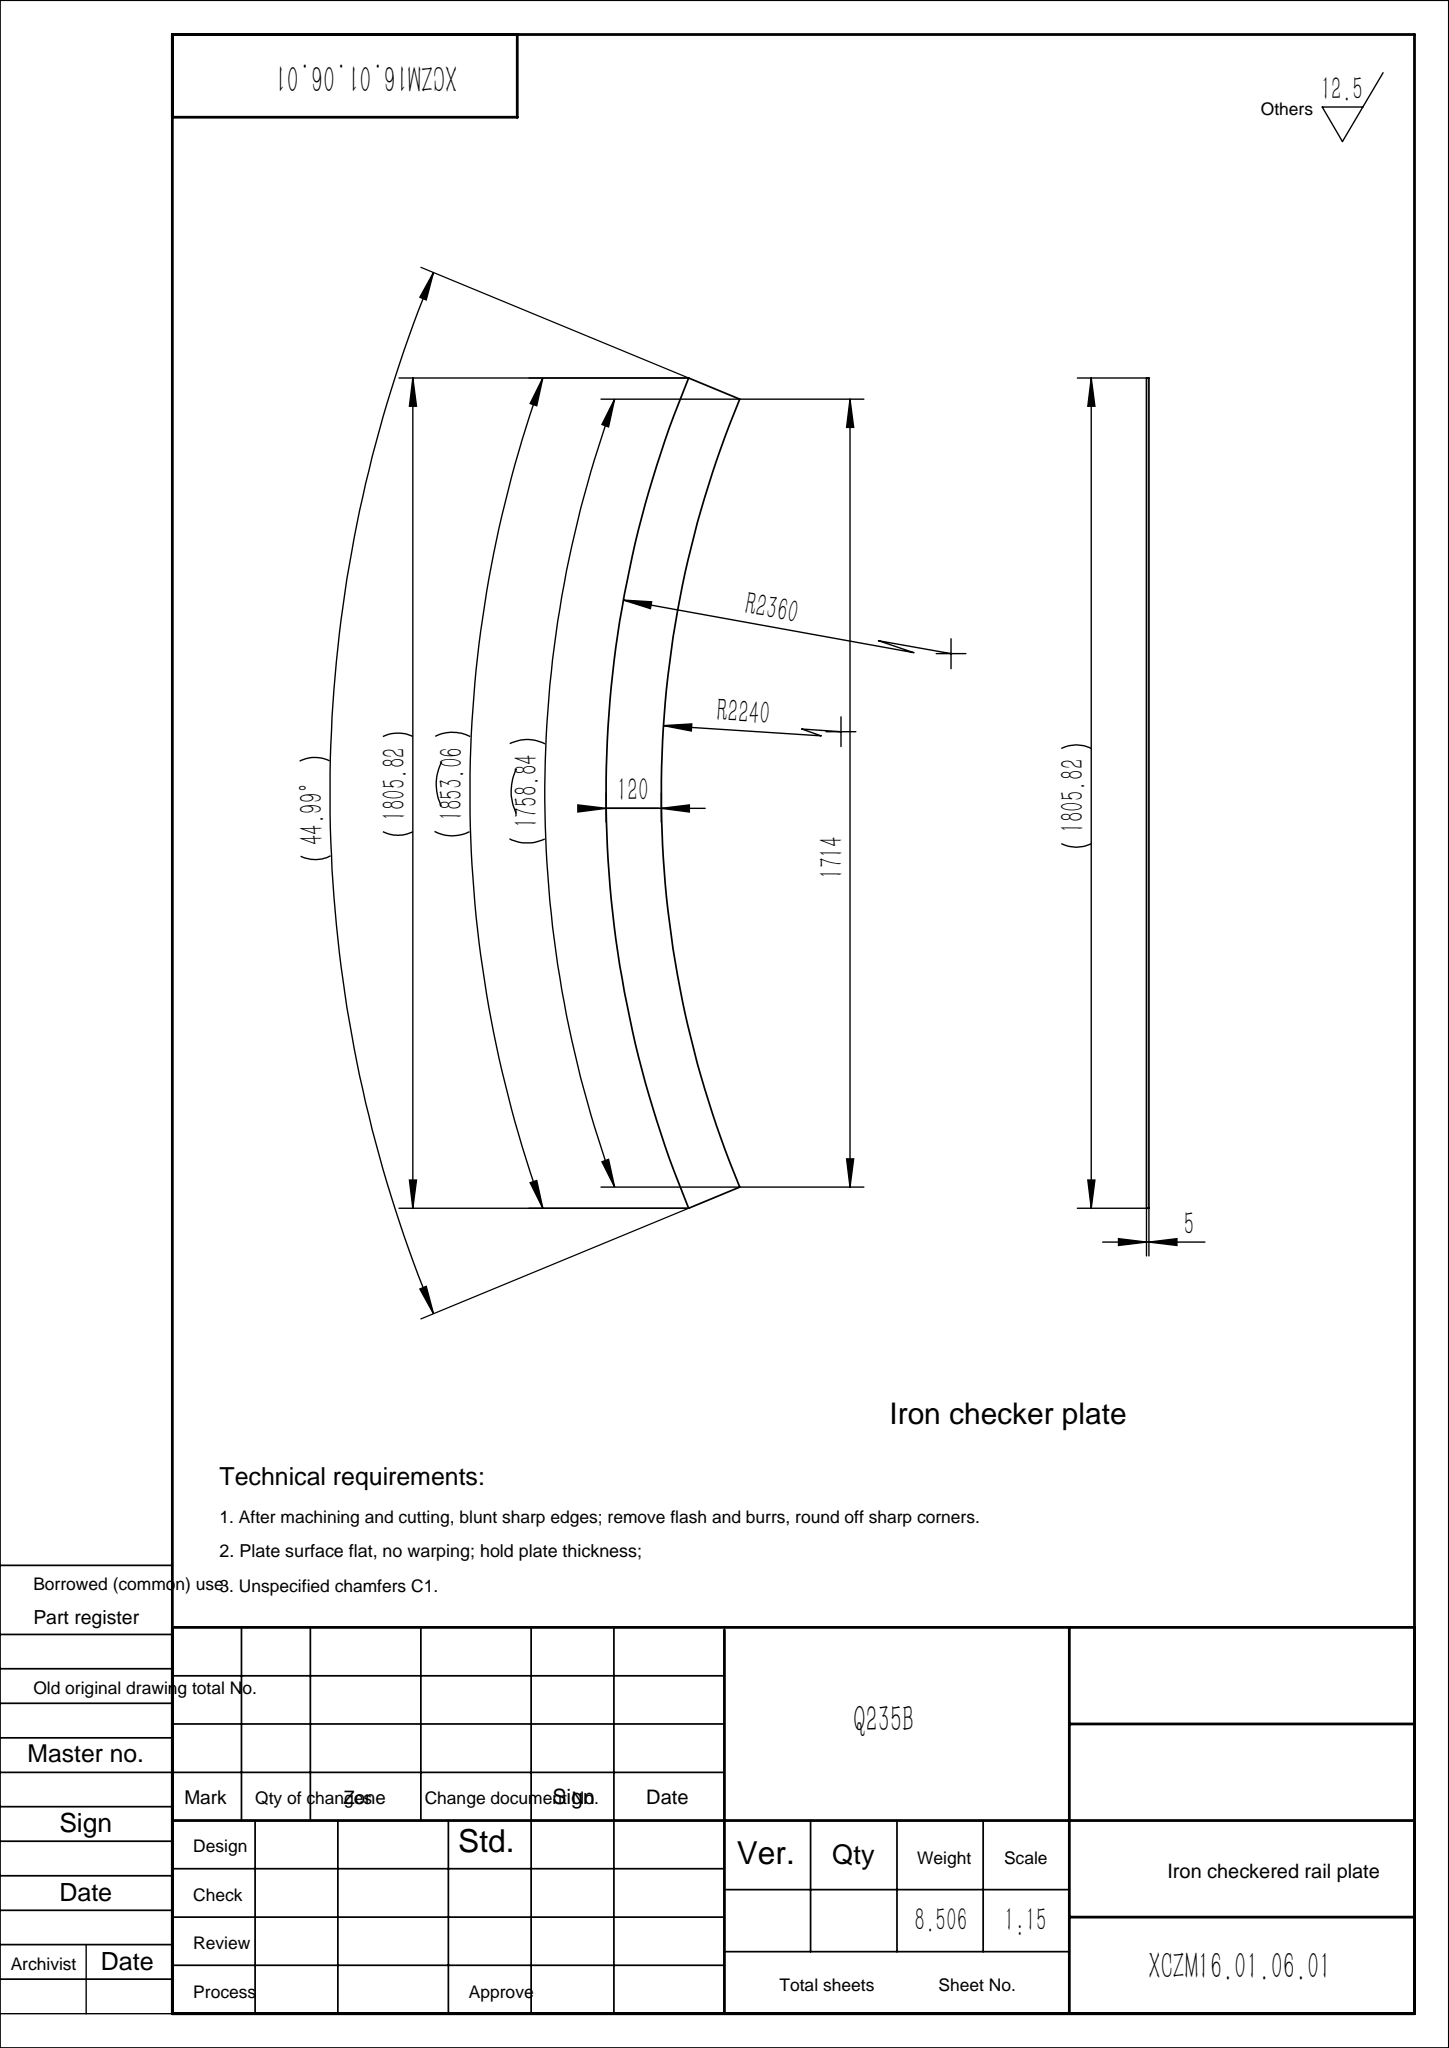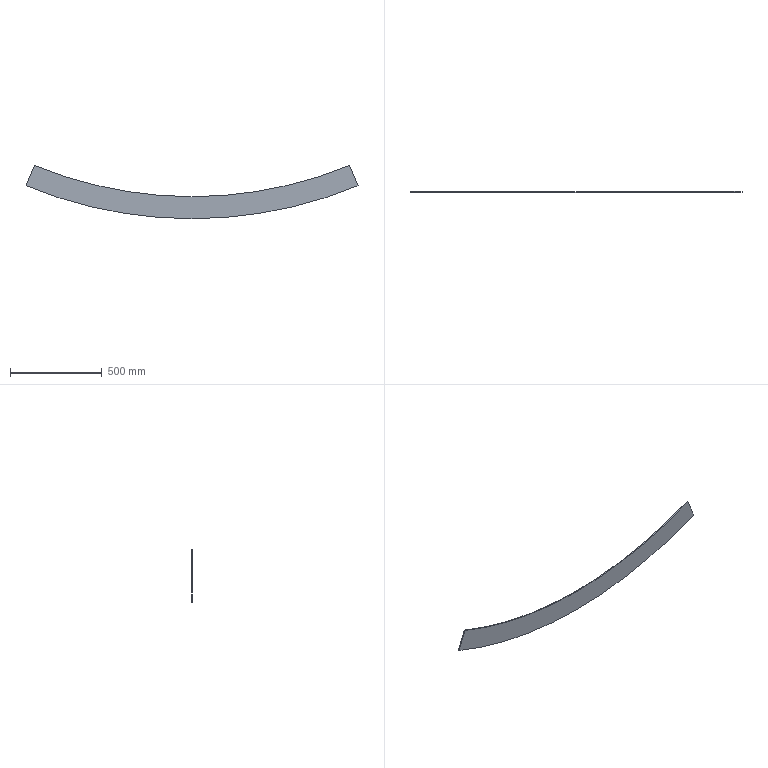Part | SolidWorks | features Extrusion 1 | 1 solid | 8 faces | box 1806 x 5 x 290.423 mm | volume 1083568 mm3 | cylinder 4 | plane 4 | commonest cylinder face diameters 4480 x2 4720 x2
STEP:
#1=CARTESIAN_POINT('',(0.,5.,-2360.));
#2=VERTEX_POINT('',#1);
#3=CARTESIAN_POINT('',(-902.911,5.,-2180.448));
#4=VERTEX_POINT('',#3);
#5=CARTESIAN_POINT('',(0.,5.,0.));
#6=DIRECTION('',(0.,1.,0.));
#7=DIRECTION('',(0.,0.,1.));
#8=AXIS2_PLACEMENT_3D('',#5,#6,#7);
#9=CIRCLE('',#8,2360.);
#10=EDGE_CURVE('',#2,#4,#9,.T.);
#11=ORIENTED_EDGE('',*,*,#10,.F.);
#12=CARTESIAN_POINT('',(0.,0.,-2360.));
#13=VERTEX_POINT('',#12);
#14=CARTESIAN_POINT('',(0.,5.,-2360.));
#15=DIRECTION('',(0.,-1.,0.));
#16=VECTOR('',#15,1000.);
#17=LINE('',#14,#16);
#18=EDGE_CURVE('',#2,#13,#17,.T.);
#19=ORIENTED_EDGE('',*,*,#18,.T.);
#20=CARTESIAN_POINT('',(-902.911,0.,-2180.448));
#21=VERTEX_POINT('',#20);
#22=CARTESIAN_POINT('',(0.,0.,0.));
#23=DIRECTION('',(0.,1.,0.));
#24=DIRECTION('',(0.,0.,1.));
#25=AXIS2_PLACEMENT_3D('',#22,#23,#24);
#26=CIRCLE('',#25,2360.);
#27=EDGE_CURVE('',#13,#21,#26,.T.);
#28=ORIENTED_EDGE('',*,*,#27,.T.);
#29=CARTESIAN_POINT('',(-902.911,5.,-2180.448));
#30=DIRECTION('',(0.,-1.,0.));
#31=VECTOR('',#30,1000.);
#32=LINE('',#29,#31);
#33=EDGE_CURVE('',#4,#21,#32,.T.);
#34=ORIENTED_EDGE('',*,*,#33,.F.);
#35=EDGE_LOOP('',(#11,#19,#28,#34));
#36=FACE_OUTER_BOUND('',#35,.T.);
#37=CARTESIAN_POINT('',(0.,5.,0.));
#38=DIRECTION('',(0.,-1.,0.));
#39=DIRECTION('',(0.,0.,-1.));
#40=AXIS2_PLACEMENT_3D('',#37,#38,#39);
#41=CYLINDRICAL_SURFACE('',#40,2360.);
#42=ADVANCED_FACE('',(#36),#41,.T.);
#43=CARTESIAN_POINT('',(857.,5.,-2069.577));
#44=VERTEX_POINT('',#43);
#45=CARTESIAN_POINT('',(0.,5.,-2240.));
#46=VERTEX_POINT('',#45);
#47=CARTESIAN_POINT('',(0.,5.,0.));
#48=DIRECTION('',(0.,1.,0.));
#49=DIRECTION('',(0.,0.,1.));
#50=AXIS2_PLACEMENT_3D('',#47,#48,#49);
#51=CIRCLE('',#50,2240.);
#52=EDGE_CURVE('',#44,#46,#51,.T.);
#53=ORIENTED_EDGE('',*,*,#52,.T.);
#54=CARTESIAN_POINT('',(0.,0.,-2240.));
#55=VERTEX_POINT('',#54);
#56=CARTESIAN_POINT('',(0.,5.,-2240.));
#57=DIRECTION('',(0.,-1.,0.));
#58=VECTOR('',#57,1000.);
#59=LINE('',#56,#58);
#60=EDGE_CURVE('',#46,#55,#59,.T.);
#61=ORIENTED_EDGE('',*,*,#60,.T.);
#62=CARTESIAN_POINT('',(857.,0.,-2069.577));
#63=VERTEX_POINT('',#62);
#64=CARTESIAN_POINT('',(0.,0.,0.));
#65=DIRECTION('',(0.,1.,0.));
#66=DIRECTION('',(0.,0.,1.));
#67=AXIS2_PLACEMENT_3D('',#64,#65,#66);
#68=CIRCLE('',#67,2240.);
#69=EDGE_CURVE('',#63,#55,#68,.T.);
#70=ORIENTED_EDGE('',*,*,#69,.F.);
#71=CARTESIAN_POINT('',(857.,5.,-2069.577));
#72=DIRECTION('',(0.,-1.,0.));
#73=VECTOR('',#72,1000.);
#74=LINE('',#71,#73);
#75=EDGE_CURVE('',#44,#63,#74,.T.);
#76=ORIENTED_EDGE('',*,*,#75,.F.);
#77=EDGE_LOOP('',(#53,#61,#70,#76));
#78=FACE_OUTER_BOUND('',#77,.T.);
#79=CARTESIAN_POINT('',(0.,5.,0.));
#80=DIRECTION('',(0.,-1.,0.));
#81=DIRECTION('',(0.,0.,-1.));
#82=AXIS2_PLACEMENT_3D('',#79,#80,#81);
#83=CYLINDRICAL_SURFACE('',#82,2240.);
#84=ADVANCED_FACE('',(#78),#83,.F.);
#85=ORIENTED_EDGE('',*,*,#60,.F.);
#86=CARTESIAN_POINT('',(-857.,5.,-2069.577));
#87=VERTEX_POINT('',#86);
#88=CARTESIAN_POINT('',(0.,5.,0.));
#89=DIRECTION('',(0.,1.,0.));
#90=DIRECTION('',(0.,0.,1.));
#91=AXIS2_PLACEMENT_3D('',#88,#89,#90);
#92=CIRCLE('',#91,2240.);
#93=EDGE_CURVE('',#46,#87,#92,.T.);
#94=ORIENTED_EDGE('',*,*,#93,.T.);
#95=CARTESIAN_POINT('',(-857.,0.,-2069.577));
#96=VERTEX_POINT('',#95);
#97=CARTESIAN_POINT('',(-857.,5.,-2069.577));
#98=DIRECTION('',(0.,-1.,0.));
#99=VECTOR('',#98,1000.);
#100=LINE('',#97,#99);
#101=EDGE_CURVE('',#87,#96,#100,.T.);
#102=ORIENTED_EDGE('',*,*,#101,.T.);
#103=CARTESIAN_POINT('',(0.,0.,0.));
#104=DIRECTION('',(0.,1.,0.));
#105=DIRECTION('',(0.,0.,1.));
#106=AXIS2_PLACEMENT_3D('',#103,#104,#105);
#107=CIRCLE('',#106,2240.);
#108=EDGE_CURVE('',#55,#96,#107,.T.);
#109=ORIENTED_EDGE('',*,*,#108,.F.);
#110=EDGE_LOOP('',(#85,#94,#102,#109));
#111=FACE_OUTER_BOUND('',#110,.T.);
#112=CARTESIAN_POINT('',(0.,5.,0.));
#113=DIRECTION('',(0.,-1.,0.));
#114=DIRECTION('',(0.,0.,-1.));
#115=AXIS2_PLACEMENT_3D('',#112,#113,#114);
#116=CYLINDRICAL_SURFACE('',#115,2240.);
#117=ADVANCED_FACE('',(#111),#116,.F.);
#118=CARTESIAN_POINT('',(902.911,0.,-2180.448));
#119=VERTEX_POINT('',#118);
#120=CARTESIAN_POINT('',(0.,0.,0.));
#121=DIRECTION('',(0.3826,0.,-0.9239));
#122=VECTOR('',#121,1000.);
#123=LINE('',#120,#122);
#124=EDGE_CURVE('',#63,#119,#123,.T.);
#125=ORIENTED_EDGE('',*,*,#124,.T.);
#126=CARTESIAN_POINT('',(902.911,5.,-2180.448));
#127=VERTEX_POINT('',#126);
#128=CARTESIAN_POINT('',(902.911,5.,-2180.448));
#129=DIRECTION('',(0.,-1.,0.));
#130=VECTOR('',#129,1000.);
#131=LINE('',#128,#130);
#132=EDGE_CURVE('',#127,#119,#131,.T.);
#133=ORIENTED_EDGE('',*,*,#132,.F.);
#134=CARTESIAN_POINT('',(0.,5.,0.));
#135=DIRECTION('',(0.3826,0.,-0.9239));
#136=VECTOR('',#135,1000.);
#137=LINE('',#134,#136);
#138=EDGE_CURVE('',#44,#127,#137,.T.);
#139=ORIENTED_EDGE('',*,*,#138,.F.);
#140=ORIENTED_EDGE('',*,*,#75,.T.);
#141=EDGE_LOOP('',(#125,#133,#139,#140));
#142=FACE_OUTER_BOUND('',#141,.T.);
#143=CARTESIAN_POINT('',(0.,5.,0.));
#144=DIRECTION('',(-0.9239,0.,-0.3826));
#145=DIRECTION('',(-0.3826,0.,0.9239));
#146=AXIS2_PLACEMENT_3D('',#143,#144,#145);
#147=PLANE('',#146);
#148=ADVANCED_FACE('',(#142),#147,.F.);
#149=ORIENTED_EDGE('',*,*,#18,.F.);
#150=CARTESIAN_POINT('',(0.,5.,0.));
#151=DIRECTION('',(0.,1.,0.));
#152=DIRECTION('',(0.,0.,1.));
#153=AXIS2_PLACEMENT_3D('',#150,#151,#152);
#154=CIRCLE('',#153,2360.);
#155=EDGE_CURVE('',#127,#2,#154,.T.);
#156=ORIENTED_EDGE('',*,*,#155,.F.);
#157=ORIENTED_EDGE('',*,*,#132,.T.);
#158=CARTESIAN_POINT('',(0.,0.,0.));
#159=DIRECTION('',(0.,1.,0.));
#160=DIRECTION('',(0.,0.,1.));
#161=AXIS2_PLACEMENT_3D('',#158,#159,#160);
#162=CIRCLE('',#161,2360.);
#163=EDGE_CURVE('',#119,#13,#162,.T.);
#164=ORIENTED_EDGE('',*,*,#163,.T.);
#165=EDGE_LOOP('',(#149,#156,#157,#164));
#166=FACE_OUTER_BOUND('',#165,.T.);
#167=CARTESIAN_POINT('',(0.,5.,0.));
#168=DIRECTION('',(0.,-1.,0.));
#169=DIRECTION('',(0.,0.,-1.));
#170=AXIS2_PLACEMENT_3D('',#167,#168,#169);
#171=CYLINDRICAL_SURFACE('',#170,2360.);
#172=ADVANCED_FACE('',(#166),#171,.T.);
#173=CARTESIAN_POINT('',(0.,0.,0.));
#174=DIRECTION('',(-0.3826,0.,-0.9239));
#175=VECTOR('',#174,1000.);
#176=LINE('',#173,#175);
#177=EDGE_CURVE('',#96,#21,#176,.T.);
#178=ORIENTED_EDGE('',*,*,#177,.F.);
#179=ORIENTED_EDGE('',*,*,#101,.F.);
#180=CARTESIAN_POINT('',(0.,5.,0.));
#181=DIRECTION('',(-0.3826,0.,-0.9239));
#182=VECTOR('',#181,1000.);
#183=LINE('',#180,#182);
#184=EDGE_CURVE('',#87,#4,#183,.T.);
#185=ORIENTED_EDGE('',*,*,#184,.T.);
#186=ORIENTED_EDGE('',*,*,#33,.T.);
#187=EDGE_LOOP('',(#178,#179,#185,#186));
#188=FACE_OUTER_BOUND('',#187,.T.);
#189=CARTESIAN_POINT('',(0.,5.,0.));
#190=DIRECTION('',(-0.9239,0.,0.3826));
#191=DIRECTION('',(0.3826,0.,0.9239));
#192=AXIS2_PLACEMENT_3D('',#189,#190,#191);
#193=PLANE('',#192);
#194=ADVANCED_FACE('',(#188),#193,.T.);
#195=ORIENTED_EDGE('',*,*,#52,.F.);
#196=ORIENTED_EDGE('',*,*,#138,.T.);
#197=ORIENTED_EDGE('',*,*,#155,.T.);
#198=ORIENTED_EDGE('',*,*,#10,.T.);
#199=ORIENTED_EDGE('',*,*,#184,.F.);
#200=ORIENTED_EDGE('',*,*,#93,.F.);
#201=EDGE_LOOP('',(#195,#196,#197,#198,#199,#200));
#202=FACE_OUTER_BOUND('',#201,.T.);
#203=CARTESIAN_POINT('',(0.,5.,0.));
#204=DIRECTION('',(0.,1.,0.));
#205=DIRECTION('',(0.,0.,1.));
#206=AXIS2_PLACEMENT_3D('',#203,#204,#205);
#207=PLANE('',#206);
#208=ADVANCED_FACE('',(#202),#207,.T.);
#209=ORIENTED_EDGE('',*,*,#69,.T.);
#210=ORIENTED_EDGE('',*,*,#108,.T.);
#211=ORIENTED_EDGE('',*,*,#177,.T.);
#212=ORIENTED_EDGE('',*,*,#27,.F.);
#213=ORIENTED_EDGE('',*,*,#163,.F.);
#214=ORIENTED_EDGE('',*,*,#124,.F.);
#215=EDGE_LOOP('',(#209,#210,#211,#212,#213,#214));
#216=FACE_OUTER_BOUND('',#215,.T.);
#217=CARTESIAN_POINT('',(0.,0.,0.));
#218=DIRECTION('',(0.,1.,0.));
#219=DIRECTION('',(0.,0.,1.));
#220=AXIS2_PLACEMENT_3D('',#217,#218,#219);
#221=PLANE('',#220);
#222=ADVANCED_FACE('',(#216),#221,.F.);
#223=CLOSED_SHELL('',(#42,#84,#117,#148,#172,#194,#208,#222));
#224=MANIFOLD_SOLID_BREP('',#223);
#225=CARTESIAN_POINT('',(0.,0.,0.));
#226=DIRECTION('',(0.,0.,1.));
#227=DIRECTION('',(1.,0.,0.));
#228=AXIS2_PLACEMENT_3D('',#225,#226,#227);
#229=(LENGTH_UNIT()NAMED_UNIT(*)SI_UNIT(.MILLI.,.METRE.));
#230=UNCERTAINTY_MEASURE_WITH_UNIT(LENGTH_MEASURE(0.00001),#229,'','');
#231=(NAMED_UNIT(*)PLANE_ANGLE_UNIT()SI_UNIT($,.RADIAN.));
#232=(NAMED_UNIT(*)SI_UNIT($,.STERADIAN.)SOLID_ANGLE_UNIT());
#233=(GEOMETRIC_REPRESENTATION_CONTEXT(3)GLOBAL_UNCERTAINTY_ASSIGNED_CONTEXT((#230))GLOBAL_UNIT_ASSIGNED_CONTEXT((#229,#231,#232))REPRESENTATION_CONTEXT('',''));
#234=ADVANCED_BREP_SHAPE_REPRESENTATION('',(#224,#228),#233);